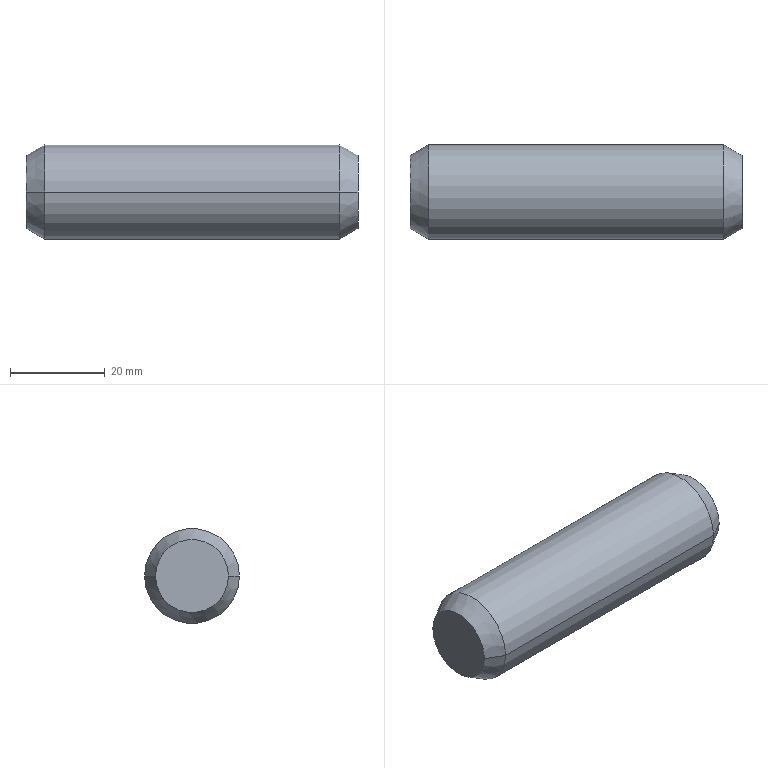Part | SolidWorks | 1 solid | 8 faces | box 70 x 20 x 20 mm | volume 21455 mm3 | cone 4 | cylinder 2 | plane 2 | commonest cylinder face diameters 20 x2
STEP:
#1=CARTESIAN_POINT('',(31.,-10.,0.));
#2=VERTEX_POINT('',#1);
#3=CARTESIAN_POINT('',(31.,10.,0.));
#4=VERTEX_POINT('',#3);
#5=CARTESIAN_POINT('',(31.,0.,0.));
#6=DIRECTION('',(-1.,0.,0.));
#7=DIRECTION('',(0.,-1.,0.));
#8=AXIS2_PLACEMENT_3D('',#5,#6,#7);
#9=CIRCLE('',#8,10.);
#10=EDGE_CURVE('',#2,#4,#9,.T.);
#11=ORIENTED_EDGE('',*,*,#10,.T.);
#12=CARTESIAN_POINT('',(-31.,10.,0.));
#13=VERTEX_POINT('',#12);
#14=CARTESIAN_POINT('',(-35.,10.,0.));
#15=DIRECTION('',(-1.,0.,0.));
#16=VECTOR('',#15,1000.);
#17=LINE('',#14,#16);
#18=EDGE_CURVE('',#4,#13,#17,.T.);
#19=ORIENTED_EDGE('',*,*,#18,.T.);
#20=CARTESIAN_POINT('',(-31.,-10.,0.));
#21=VERTEX_POINT('',#20);
#22=CARTESIAN_POINT('',(-31.,0.,0.));
#23=DIRECTION('',(-1.,0.,0.));
#24=DIRECTION('',(0.,-1.,0.));
#25=AXIS2_PLACEMENT_3D('',#22,#23,#24);
#26=CIRCLE('',#25,10.);
#27=EDGE_CURVE('',#21,#13,#26,.T.);
#28=ORIENTED_EDGE('',*,*,#27,.F.);
#29=CARTESIAN_POINT('',(-35.,-10.,0.));
#30=DIRECTION('',(-1.,0.,0.));
#31=VECTOR('',#30,1000.);
#32=LINE('',#29,#31);
#33=EDGE_CURVE('',#2,#21,#32,.T.);
#34=ORIENTED_EDGE('',*,*,#33,.F.);
#35=EDGE_LOOP('',(#11,#19,#28,#34));
#36=FACE_OUTER_BOUND('',#35,.T.);
#37=CARTESIAN_POINT('',(-35.,0.,0.));
#38=DIRECTION('',(-1.,0.,0.));
#39=DIRECTION('',(0.,-1.,0.));
#40=AXIS2_PLACEMENT_3D('',#37,#38,#39);
#41=CYLINDRICAL_SURFACE('',#40,10.);
#42=ADVANCED_FACE('',(#36),#41,.T.);
#43=CARTESIAN_POINT('',(35.,-7.691,0.));
#44=VERTEX_POINT('',#43);
#45=CARTESIAN_POINT('',(35.,7.691,0.));
#46=VERTEX_POINT('',#45);
#47=CARTESIAN_POINT('',(35.,0.,0.));
#48=DIRECTION('',(-1.,0.,0.));
#49=DIRECTION('',(0.,-1.,0.));
#50=AXIS2_PLACEMENT_3D('',#47,#48,#49);
#51=CIRCLE('',#50,7.691);
#52=EDGE_CURVE('',#44,#46,#51,.T.);
#53=ORIENTED_EDGE('',*,*,#52,.T.);
#54=CARTESIAN_POINT('',(35.,7.691,0.));
#55=DIRECTION('',(-0.866,0.5,0.));
#56=VECTOR('',#55,1000.);
#57=LINE('',#54,#56);
#58=EDGE_CURVE('',#46,#4,#57,.T.);
#59=ORIENTED_EDGE('',*,*,#58,.T.);
#60=ORIENTED_EDGE('',*,*,#10,.F.);
#61=CARTESIAN_POINT('',(35.,-7.691,0.));
#62=DIRECTION('',(-0.866,-0.5,0.));
#63=VECTOR('',#62,1000.);
#64=LINE('',#61,#63);
#65=EDGE_CURVE('',#44,#2,#64,.T.);
#66=ORIENTED_EDGE('',*,*,#65,.F.);
#67=EDGE_LOOP('',(#53,#59,#60,#66));
#68=FACE_OUTER_BOUND('',#67,.T.);
#69=CARTESIAN_POINT('',(35.,0.,0.));
#70=DIRECTION('',(-1.,0.,0.));
#71=DIRECTION('',(0.,-1.,0.));
#72=AXIS2_PLACEMENT_3D('',#69,#70,#71);
#73=CONICAL_SURFACE('',#72,7.691,0.5236);
#74=ADVANCED_FACE('',(#68),#73,.T.);
#75=CARTESIAN_POINT('',(-35.,-7.691,0.));
#76=VERTEX_POINT('',#75);
#77=CARTESIAN_POINT('',(-35.,7.691,0.));
#78=VERTEX_POINT('',#77);
#79=CARTESIAN_POINT('',(-35.,0.,0.));
#80=DIRECTION('',(-1.,0.,0.));
#81=DIRECTION('',(0.,-1.,0.));
#82=AXIS2_PLACEMENT_3D('',#79,#80,#81);
#83=CIRCLE('',#82,7.691);
#84=EDGE_CURVE('',#76,#78,#83,.T.);
#85=ORIENTED_EDGE('',*,*,#84,.F.);
#86=CARTESIAN_POINT('',(-31.,-10.,0.));
#87=DIRECTION('',(0.866,-0.5,0.));
#88=VECTOR('',#87,1000.);
#89=LINE('',#86,#88);
#90=EDGE_CURVE('',#76,#21,#89,.T.);
#91=ORIENTED_EDGE('',*,*,#90,.T.);
#92=ORIENTED_EDGE('',*,*,#27,.T.);
#93=CARTESIAN_POINT('',(-31.,10.,0.));
#94=DIRECTION('',(0.866,0.5,0.));
#95=VECTOR('',#94,1000.);
#96=LINE('',#93,#95);
#97=EDGE_CURVE('',#78,#13,#96,.T.);
#98=ORIENTED_EDGE('',*,*,#97,.F.);
#99=EDGE_LOOP('',(#85,#91,#92,#98));
#100=FACE_OUTER_BOUND('',#99,.T.);
#101=CARTESIAN_POINT('',(-31.,0.,0.));
#102=DIRECTION('',(1.,0.,0.));
#103=DIRECTION('',(0.,1.,0.));
#104=AXIS2_PLACEMENT_3D('',#101,#102,#103);
#105=CONICAL_SURFACE('',#104,10.,0.5236);
#106=ADVANCED_FACE('',(#100),#105,.T.);
#107=ORIENTED_EDGE('',*,*,#90,.F.);
#108=CARTESIAN_POINT('',(-35.,0.,0.));
#109=DIRECTION('',(-1.,0.,0.));
#110=DIRECTION('',(0.,-1.,0.));
#111=AXIS2_PLACEMENT_3D('',#108,#109,#110);
#112=CIRCLE('',#111,7.691);
#113=EDGE_CURVE('',#78,#76,#112,.T.);
#114=ORIENTED_EDGE('',*,*,#113,.F.);
#115=ORIENTED_EDGE('',*,*,#97,.T.);
#116=CARTESIAN_POINT('',(-31.,0.,0.));
#117=DIRECTION('',(-1.,0.,0.));
#118=DIRECTION('',(0.,-1.,0.));
#119=AXIS2_PLACEMENT_3D('',#116,#117,#118);
#120=CIRCLE('',#119,10.);
#121=EDGE_CURVE('',#13,#21,#120,.T.);
#122=ORIENTED_EDGE('',*,*,#121,.T.);
#123=EDGE_LOOP('',(#107,#114,#115,#122));
#124=FACE_OUTER_BOUND('',#123,.T.);
#125=CARTESIAN_POINT('',(-31.,0.,0.));
#126=DIRECTION('',(1.,0.,0.));
#127=DIRECTION('',(0.,1.,0.));
#128=AXIS2_PLACEMENT_3D('',#125,#126,#127);
#129=CONICAL_SURFACE('',#128,10.,0.5236);
#130=ADVANCED_FACE('',(#124),#129,.T.);
#131=ORIENTED_EDGE('',*,*,#113,.T.);
#132=ORIENTED_EDGE('',*,*,#84,.T.);
#133=EDGE_LOOP('',(#131,#132));
#134=FACE_OUTER_BOUND('',#133,.T.);
#135=CARTESIAN_POINT('',(-35.,7.691,0.));
#136=DIRECTION('',(1.,0.,0.));
#137=DIRECTION('',(0.,1.,0.));
#138=AXIS2_PLACEMENT_3D('',#135,#136,#137);
#139=PLANE('',#138);
#140=ADVANCED_FACE('',(#134),#139,.F.);
#141=ORIENTED_EDGE('',*,*,#52,.F.);
#142=CARTESIAN_POINT('',(35.,0.,0.));
#143=DIRECTION('',(-1.,0.,0.));
#144=DIRECTION('',(0.,-1.,0.));
#145=AXIS2_PLACEMENT_3D('',#142,#143,#144);
#146=CIRCLE('',#145,7.691);
#147=EDGE_CURVE('',#46,#44,#146,.T.);
#148=ORIENTED_EDGE('',*,*,#147,.F.);
#149=EDGE_LOOP('',(#141,#148));
#150=FACE_OUTER_BOUND('',#149,.T.);
#151=CARTESIAN_POINT('',(35.,7.691,0.));
#152=DIRECTION('',(-1.,0.,0.));
#153=DIRECTION('',(0.,-1.,0.));
#154=AXIS2_PLACEMENT_3D('',#151,#152,#153);
#155=PLANE('',#154);
#156=ADVANCED_FACE('',(#150),#155,.F.);
#157=ORIENTED_EDGE('',*,*,#58,.F.);
#158=ORIENTED_EDGE('',*,*,#147,.T.);
#159=ORIENTED_EDGE('',*,*,#65,.T.);
#160=CARTESIAN_POINT('',(31.,0.,0.));
#161=DIRECTION('',(-1.,0.,0.));
#162=DIRECTION('',(0.,-1.,0.));
#163=AXIS2_PLACEMENT_3D('',#160,#161,#162);
#164=CIRCLE('',#163,10.);
#165=EDGE_CURVE('',#4,#2,#164,.T.);
#166=ORIENTED_EDGE('',*,*,#165,.F.);
#167=EDGE_LOOP('',(#157,#158,#159,#166));
#168=FACE_OUTER_BOUND('',#167,.T.);
#169=CARTESIAN_POINT('',(35.,0.,0.));
#170=DIRECTION('',(-1.,0.,0.));
#171=DIRECTION('',(0.,-1.,0.));
#172=AXIS2_PLACEMENT_3D('',#169,#170,#171);
#173=CONICAL_SURFACE('',#172,7.691,0.5236);
#174=ADVANCED_FACE('',(#168),#173,.T.);
#175=ORIENTED_EDGE('',*,*,#18,.F.);
#176=ORIENTED_EDGE('',*,*,#165,.T.);
#177=ORIENTED_EDGE('',*,*,#33,.T.);
#178=ORIENTED_EDGE('',*,*,#121,.F.);
#179=EDGE_LOOP('',(#175,#176,#177,#178));
#180=FACE_OUTER_BOUND('',#179,.T.);
#181=CARTESIAN_POINT('',(-35.,0.,0.));
#182=DIRECTION('',(-1.,0.,0.));
#183=DIRECTION('',(0.,-1.,0.));
#184=AXIS2_PLACEMENT_3D('',#181,#182,#183);
#185=CYLINDRICAL_SURFACE('',#184,10.);
#186=ADVANCED_FACE('',(#180),#185,.T.);
#187=CLOSED_SHELL('',(#42,#74,#106,#130,#140,#156,#174,#186));
#188=MANIFOLD_SOLID_BREP('',#187);
#189=CARTESIAN_POINT('',(0.,0.,0.));
#190=DIRECTION('',(0.,0.,1.));
#191=DIRECTION('',(1.,0.,0.));
#192=AXIS2_PLACEMENT_3D('',#189,#190,#191);
#193=(LENGTH_UNIT()NAMED_UNIT(*)SI_UNIT(.MILLI.,.METRE.));
#194=UNCERTAINTY_MEASURE_WITH_UNIT(LENGTH_MEASURE(0.00001),#193,'','');
#195=(NAMED_UNIT(*)PLANE_ANGLE_UNIT()SI_UNIT($,.RADIAN.));
#196=(NAMED_UNIT(*)SI_UNIT($,.STERADIAN.)SOLID_ANGLE_UNIT());
#197=(GEOMETRIC_REPRESENTATION_CONTEXT(3)GLOBAL_UNCERTAINTY_ASSIGNED_CONTEXT((#194))GLOBAL_UNIT_ASSIGNED_CONTEXT((#193,#195,#196))REPRESENTATION_CONTEXT('',''));
#198=ADVANCED_BREP_SHAPE_REPRESENTATION('',(#188,#192),#197);